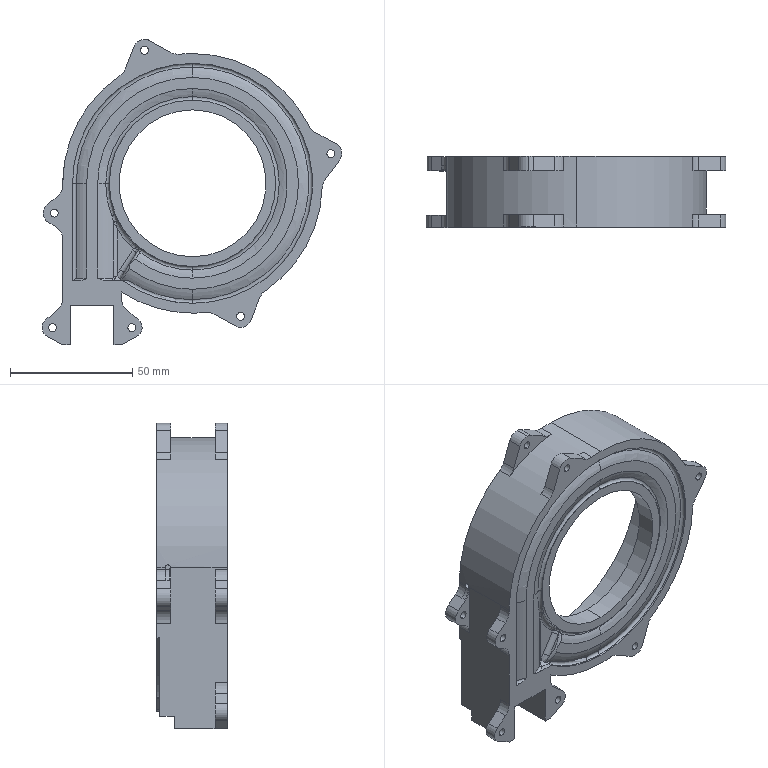Part | SolidWorks | features ICE 18, Fillet 13, Extrusion 1, Shell 1, SweepCut 1 | 1 solid | 217 faces | box 122.366 x 28.8 x 124.721 mm | volume 74874 mm3 | cylinder 104 | plane 68 | torus 26 | spline 19 | commonest cylinder face diameters 12 x22 3.2 x20 9 x10 4 x7 2.1 x4 5 x4